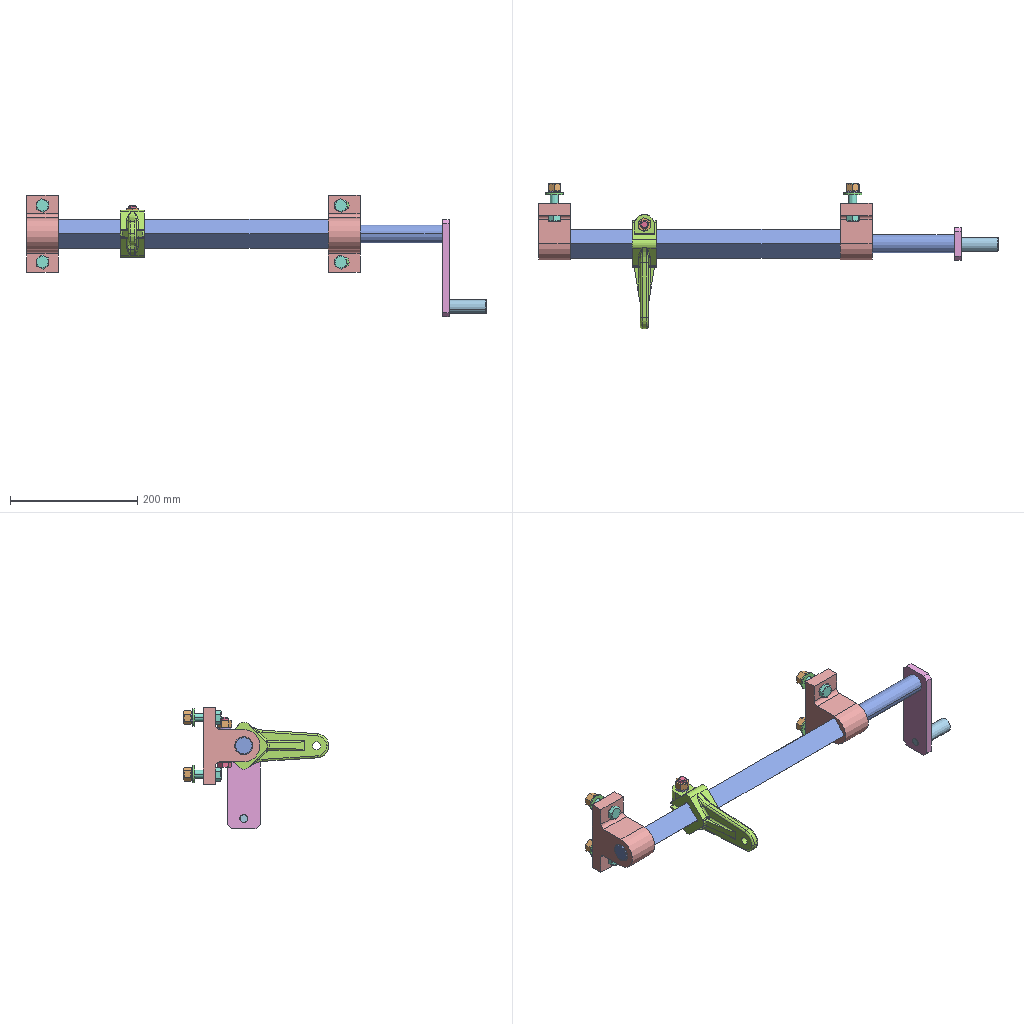Assembly | SolidWorks | 10 different items | 25 placed | box 723 x 229 x 191 mm
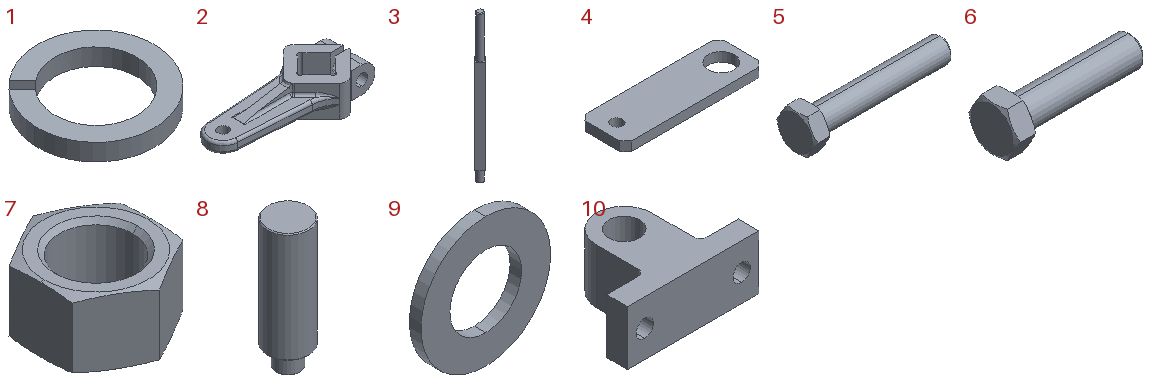Parts list (item | quantity | size | volume | features):
1 | x5 | 20.15 x 20.15 x 4.655 mm | 458.797 mm3 | features Boss 1, Cut 1, Extrusion 1, Helix 1, Sweep 1
2 | x1 | 179.388 x 74.009 x 38.1 mm | 152427 mm3 | features Fillet 4, Cut 3, MirrorPattern 2, Boss 1, Extrusion 1, Rib 1
3 | x1 | 45.255 x 45.255 x 664.7 mm | 588102 mm3 | features Chamfer 2, Extrusion 1, RevCut 1
4 | x1 | 152.4 x 50.8 x 10 mm | 68933 mm3 | features Chamfer 1, Extrusion 1
5 | x1 | 78.581 x 21.997 x 19.05 mm | 11501 mm3 | features RevCut 4, Chamfer 1, Extrusion 1, Fillet 1, LPattern 1, Revolution 1
6 | x4 | 59.531 x 21.997 x 19.05 mm | 9087 mm3 | features RevCut 4, Chamfer 1, Extrusion 1, Fillet 1, LPattern 1, Revolution 1
7 | x5 | 19.096 x 22 x 11.38 mm | 2097 mm3 | features Cut 2, Chamfer 1, Extrusion 1
8 | x1 | 22 x 22 x 68 mm | 23293 mm3 | features Chamfer 1, Extrusion 1, ICE 1
9 | x4 | 28 x 2.5 x 28 mm | 1068 mm3 | features Revolution 1
10 | x2 | 120.65 x 88.9 x 50 mm | 239631 mm3 | features Cut 1, Extrusion 1, Fillet 1
Mates (type | each side: item.copy, entity, surface, feature):
Coincident | 10.1 plane | assembly plane | 3 times
Concentric | 10.1 face cylinder Extrude1 | 3.1 face cylinder Cut-Revolve1
Coincident | 10.1 face plane Extrude1 | 3.1 face plane Cut-Revolve1
Concentric | 3.1 face cylinder Cut-Revolve1 | 10.2 face cylinder Extrude1
Coincident | 3.1 face plane Cut-Revolve1 | 10.2 face plane Extrude1
Coincident | 10.1 face plane Extrude1 | 10.2 face plane Extrude1
Coincident | 3.1 plane | 2.1 plane | 2 times
Concentric | 3.1 face cylinder Cut-Revolve1 | 4.1 face cylinder Extrude1
Coincident | 3.1 face plane Extrude1 | 4.1 face plane Extrude1
Perpendicular | 2.1 plane | 4.1 plane
Coincident | 2.1 plane | assembly plane
DistanceDim | 2.1 plane | assembly plane
Concentric | 10.1 face cylinder Cut-Extrude1 | 6.1 face cylinder Boss-Revolve1
Concentric | 6.1 face cylinder Boss-Revolve1 | 9.1 face cylinder Base-Revolve
Coincident | 10.1 face plane Extrude1 | 6.1 face plane Base-Extrude
Concentric | 6.1 face cylinder Boss-Revolve1 | 1.1 face cylinder Boss-Extrude1
Concentric | 6.1 face cylinder Boss-Revolve1 | 7.1 face cylinder Base-Extrude
Coincident | 1.1 face plane Base-Extrude | 7.1 face plane Base-Extrude
Coincident | 9.1 face plane Base-Revolve | 1.1 face plane Boss-Extrude1
Concentric | 2.1 face cylinder Cut-Extrude2 | 5.1 face cylinder Boss-Revolve1
Coincident | 2.1 face plane Extrude2 | 5.1 face plane Base-Extrude
Concentric | 5.1 face cylinder Boss-Revolve1 | 9.2 face
Concentric | 5.1 face cylinder Boss-Revolve1 | 1.2 face cylinder Boss-Extrude1
Concentric | 5.1 face cylinder Boss-Revolve1 | 7.2 face cylinder Base-Extrude
Coincident | 2.1 face plane Extrude2 | 9.2 face
Coincident | 1.2 face plane Boss-Extrude1 | 2.1 face plane Extrude2
Coincident | 1.2 face plane Base-Extrude | 7.2 face plane Base-Extrude
Concentric | 4.1 face cylinder Extrude1 | 8.1 face cylinder Boss-Extrude1
Coincident | 4.1 face plane Extrude1 | 8.1 face plane Boss-Extrude2